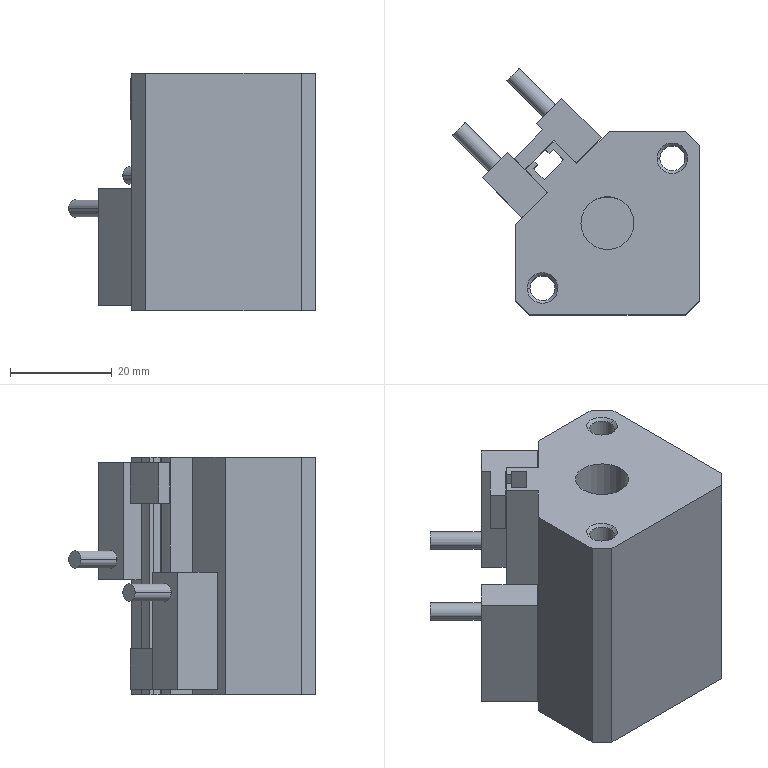Part | STEP file | CDQ2A20_15D_F7NV0 | 1 solid | 73 faces | box 48.335 x 48.335 x 46.5 mm | volume 53480 mm3 | plane 47 | cylinder 14 | cone 12 | commonest cylinder face diameters 3.4 x4 4.13 x4 4.92 x4 10.4 x2